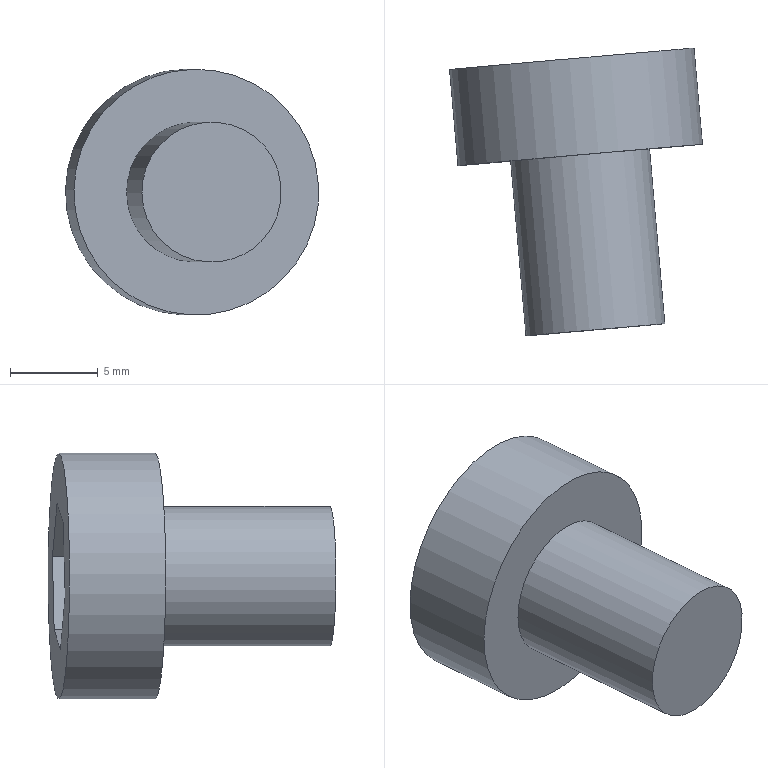Part | NX | features solid 2 | 1 solid | 12 faces | box 14.426 x 16.398 x 14 mm | volume 1177 mm3 | plane 10 | spline 1 | cylinder 1 | commonest cylinder face diameters 14 x1